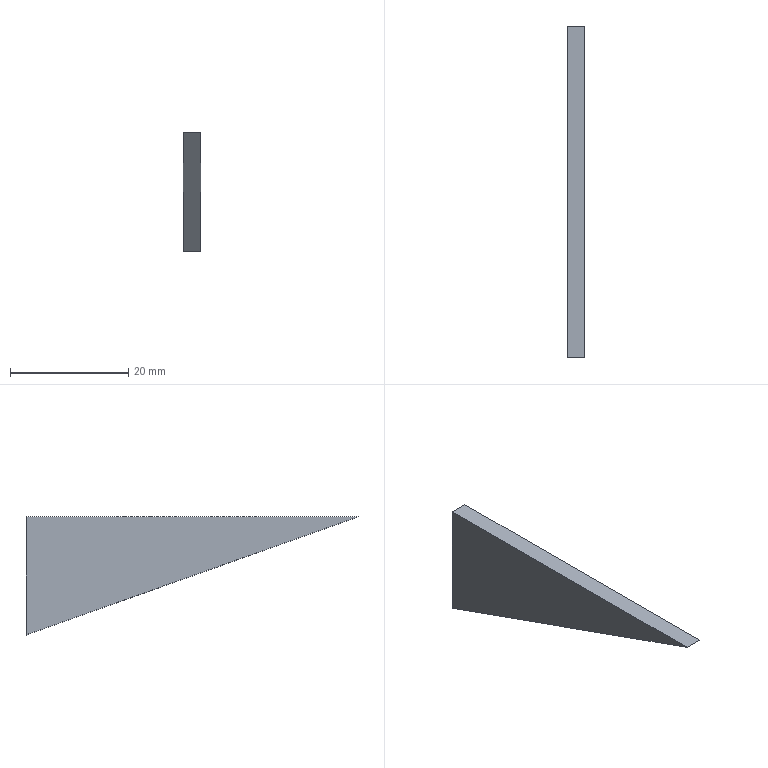Part | STEP file | 1 solid | 5 faces | box 3 x 56.217 x 20 mm | volume 1687 mm3 | plane 5
STEP:
#1=CARTESIAN_POINT('',(0.,0.,0.));
#2=DIRECTION('',(0.,0.,1.));
#3=DIRECTION('',(1.,0.,0.));
#4=AXIS2_PLACEMENT_3D('',#1,#2,#3);
#5=CARTESIAN_POINT('',(365.177,734.79,117.013));
#6=VERTEX_POINT('',#5);
#7=CARTESIAN_POINT('',(365.177,734.79,137.013));
#8=VERTEX_POINT('',#7);
#9=CARTESIAN_POINT('',(365.177,734.79,137.013));
#10=DIRECTION('',(0.,0.,1.));
#11=VECTOR('',#10,1.);
#12=LINE('',#9,#11);
#13=CARTESIAN_POINT('',(362.177,734.79,137.013));
#14=DIRECTION('',(0.,1.,0.));
#15=DIRECTION('',(0.,0.,1.));
#16=AXIS2_PLACEMENT_3D('',#13,#14,#15);
#17=PLANE('',#16);
#18=CARTESIAN_POINT('',(0.,3.));
#19=DIRECTION('',(1.,0.));
#20=VECTOR('',#19,1.);
#21=LINE('',#18,#20);
#22=(GEOMETRIC_REPRESENTATION_CONTEXT(2)PARAMETRIC_REPRESENTATION_CONTEXT()REPRESENTATION_CONTEXT('',''));
#23=DEFINITIONAL_REPRESENTATION('',(#21),#22);
#24=PCURVE('',#17,#23);
#25=CARTESIAN_POINT('',(365.177,0.,0.));
#26=DIRECTION('',(1.,0.,0.));
#27=DIRECTION('',(0.,0.,-1.));
#28=AXIS2_PLACEMENT_3D('',#25,#26,#27);
#29=PLANE('',#28);
#30=CARTESIAN_POINT('',(-137.013,734.79));
#31=DIRECTION('',(-1.,0.));
#32=VECTOR('',#31,1.);
#33=LINE('',#30,#32);
#34=(GEOMETRIC_REPRESENTATION_CONTEXT(2)PARAMETRIC_REPRESENTATION_CONTEXT()REPRESENTATION_CONTEXT('',''));
#35=DEFINITIONAL_REPRESENTATION('',(#33),#34);
#36=PCURVE('',#29,#35);
#37=SURFACE_CURVE('',#12,(#24,#36),.PCURVE_S1.);
#38=EDGE_CURVE('',#6,#8,#37,.T.);
#39=ORIENTED_EDGE('',*,*,#38,.F.);
#40=CARTESIAN_POINT('',(362.177,734.79,117.013));
#41=VERTEX_POINT('',#40);
#42=CARTESIAN_POINT('',(362.177,734.79,117.013));
#43=DIRECTION('',(1.,0.,0.));
#44=VECTOR('',#43,1.);
#45=LINE('',#42,#44);
#46=CARTESIAN_POINT('',(-20.,0.));
#47=DIRECTION('',(0.,1.));
#48=VECTOR('',#47,1.);
#49=LINE('',#46,#48);
#50=(GEOMETRIC_REPRESENTATION_CONTEXT(2)PARAMETRIC_REPRESENTATION_CONTEXT()REPRESENTATION_CONTEXT('',''));
#51=DEFINITIONAL_REPRESENTATION('',(#49),#50);
#52=PCURVE('',#17,#51);
#53=CARTESIAN_POINT('',(362.177,734.79,117.013));
#54=DIRECTION('',(0.,-0.3352,-0.9422));
#55=DIRECTION('',(0.,0.9422,-0.3352));
#56=AXIS2_PLACEMENT_3D('',#53,#54,#55);
#57=PLANE('',#56);
#58=CARTESIAN_POINT('',(0.,0.));
#59=DIRECTION('',(0.,1.));
#60=VECTOR('',#59,1.);
#61=LINE('',#58,#60);
#62=(GEOMETRIC_REPRESENTATION_CONTEXT(2)PARAMETRIC_REPRESENTATION_CONTEXT()REPRESENTATION_CONTEXT('',''));
#63=DEFINITIONAL_REPRESENTATION('',(#61),#62);
#64=PCURVE('',#57,#63);
#65=SURFACE_CURVE('',#45,(#52,#64),.PCURVE_S1.);
#66=EDGE_CURVE('',#41,#6,#65,.T.);
#67=ORIENTED_EDGE('',*,*,#66,.F.);
#68=CARTESIAN_POINT('',(362.177,734.79,137.013));
#69=VERTEX_POINT('',#68);
#70=CARTESIAN_POINT('',(362.177,734.79,137.013));
#71=DIRECTION('',(0.,0.,1.));
#72=VECTOR('',#71,1.);
#73=LINE('',#70,#72);
#74=CARTESIAN_POINT('',(0.,0.));
#75=DIRECTION('',(1.,0.));
#76=VECTOR('',#75,1.);
#77=LINE('',#74,#76);
#78=(GEOMETRIC_REPRESENTATION_CONTEXT(2)PARAMETRIC_REPRESENTATION_CONTEXT()REPRESENTATION_CONTEXT('',''));
#79=DEFINITIONAL_REPRESENTATION('',(#77),#78);
#80=PCURVE('',#17,#79);
#81=CARTESIAN_POINT('',(362.177,0.,0.));
#82=DIRECTION('',(1.,0.,0.));
#83=DIRECTION('',(0.,0.,-1.));
#84=AXIS2_PLACEMENT_3D('',#81,#82,#83);
#85=PLANE('',#84);
#86=CARTESIAN_POINT('',(-137.013,734.79));
#87=DIRECTION('',(-1.,0.));
#88=VECTOR('',#87,1.);
#89=LINE('',#86,#88);
#90=(GEOMETRIC_REPRESENTATION_CONTEXT(2)PARAMETRIC_REPRESENTATION_CONTEXT()REPRESENTATION_CONTEXT('',''));
#91=DEFINITIONAL_REPRESENTATION('',(#89),#90);
#92=PCURVE('',#85,#91);
#93=SURFACE_CURVE('',#73,(#80,#92),.PCURVE_S1.);
#94=EDGE_CURVE('',#41,#69,#93,.T.);
#95=ORIENTED_EDGE('',*,*,#94,.T.);
#96=CARTESIAN_POINT('',(362.177,734.79,137.013));
#97=DIRECTION('',(1.,0.,0.));
#98=VECTOR('',#97,1.);
#99=LINE('',#96,#98);
#100=CARTESIAN_POINT('',(0.,0.));
#101=DIRECTION('',(0.,1.));
#102=VECTOR('',#101,1.);
#103=LINE('',#100,#102);
#104=(GEOMETRIC_REPRESENTATION_CONTEXT(2)PARAMETRIC_REPRESENTATION_CONTEXT()REPRESENTATION_CONTEXT('',''));
#105=DEFINITIONAL_REPRESENTATION('',(#103),#104);
#106=PCURVE('',#17,#105);
#107=CARTESIAN_POINT('',(362.177,678.573,137.013));
#108=DIRECTION('',(0.,0.,1.));
#109=DIRECTION('',(1.,0.,0.));
#110=AXIS2_PLACEMENT_3D('',#107,#108,#109);
#111=PLANE('',#110);
#112=CARTESIAN_POINT('',(0.,56.217));
#113=DIRECTION('',(1.,0.));
#114=VECTOR('',#113,1.);
#115=LINE('',#112,#114);
#116=(GEOMETRIC_REPRESENTATION_CONTEXT(2)PARAMETRIC_REPRESENTATION_CONTEXT()REPRESENTATION_CONTEXT('',''));
#117=DEFINITIONAL_REPRESENTATION('',(#115),#116);
#118=PCURVE('',#111,#117);
#119=SURFACE_CURVE('',#99,(#106,#118),.PCURVE_S1.);
#120=EDGE_CURVE('',#69,#8,#119,.T.);
#121=ORIENTED_EDGE('',*,*,#120,.T.);
#122=EDGE_LOOP('',(#39,#67,#95,#121));
#123=FACE_BOUND('',#122,.T.);
#124=ADVANCED_FACE('',(#123),#17,.T.);
#125=CARTESIAN_POINT('',(365.177,678.573,137.013));
#126=VERTEX_POINT('',#125);
#127=CARTESIAN_POINT('',(365.177,734.79,117.013));
#128=DIRECTION('',(0.,0.9422,-0.3352));
#129=VECTOR('',#128,1.);
#130=LINE('',#127,#129);
#131=CARTESIAN_POINT('',(0.,3.));
#132=DIRECTION('',(1.,0.));
#133=VECTOR('',#132,1.);
#134=LINE('',#131,#133);
#135=(GEOMETRIC_REPRESENTATION_CONTEXT(2)PARAMETRIC_REPRESENTATION_CONTEXT()REPRESENTATION_CONTEXT('',''));
#136=DEFINITIONAL_REPRESENTATION('',(#134),#135);
#137=PCURVE('',#57,#136);
#138=CARTESIAN_POINT('',(-117.013,734.79));
#139=DIRECTION('',(0.3352,0.9422));
#140=VECTOR('',#139,1.);
#141=LINE('',#138,#140);
#142=(GEOMETRIC_REPRESENTATION_CONTEXT(2)PARAMETRIC_REPRESENTATION_CONTEXT()REPRESENTATION_CONTEXT('',''));
#143=DEFINITIONAL_REPRESENTATION('',(#141),#142);
#144=PCURVE('',#29,#143);
#145=SURFACE_CURVE('',#130,(#137,#144),.PCURVE_S1.);
#146=EDGE_CURVE('',#126,#6,#145,.T.);
#147=ORIENTED_EDGE('',*,*,#146,.F.);
#148=CARTESIAN_POINT('',(362.177,678.573,137.013));
#149=VERTEX_POINT('',#148);
#150=CARTESIAN_POINT('',(362.177,678.573,137.013));
#151=DIRECTION('',(1.,0.,0.));
#152=VECTOR('',#151,1.);
#153=LINE('',#150,#152);
#154=CARTESIAN_POINT('',(-59.669,0.));
#155=DIRECTION('',(0.,1.));
#156=VECTOR('',#155,1.);
#157=LINE('',#154,#156);
#158=(GEOMETRIC_REPRESENTATION_CONTEXT(2)PARAMETRIC_REPRESENTATION_CONTEXT()REPRESENTATION_CONTEXT('',''));
#159=DEFINITIONAL_REPRESENTATION('',(#157),#158);
#160=PCURVE('',#57,#159);
#161=CARTESIAN_POINT('',(0.,0.));
#162=DIRECTION('',(1.,0.));
#163=VECTOR('',#162,1.);
#164=LINE('',#161,#163);
#165=(GEOMETRIC_REPRESENTATION_CONTEXT(2)PARAMETRIC_REPRESENTATION_CONTEXT()REPRESENTATION_CONTEXT('',''));
#166=DEFINITIONAL_REPRESENTATION('',(#164),#165);
#167=PCURVE('',#111,#166);
#168=SURFACE_CURVE('',#153,(#160,#167),.PCURVE_S1.);
#169=EDGE_CURVE('',#149,#126,#168,.T.);
#170=ORIENTED_EDGE('',*,*,#169,.F.);
#171=CARTESIAN_POINT('',(362.177,734.79,117.013));
#172=DIRECTION('',(0.,0.9422,-0.3352));
#173=VECTOR('',#172,1.);
#174=LINE('',#171,#173);
#175=CARTESIAN_POINT('',(0.,0.));
#176=DIRECTION('',(1.,0.));
#177=VECTOR('',#176,1.);
#178=LINE('',#175,#177);
#179=(GEOMETRIC_REPRESENTATION_CONTEXT(2)PARAMETRIC_REPRESENTATION_CONTEXT()REPRESENTATION_CONTEXT('',''));
#180=DEFINITIONAL_REPRESENTATION('',(#178),#179);
#181=PCURVE('',#57,#180);
#182=CARTESIAN_POINT('',(-117.013,734.79));
#183=DIRECTION('',(0.3352,0.9422));
#184=VECTOR('',#183,1.);
#185=LINE('',#182,#184);
#186=(GEOMETRIC_REPRESENTATION_CONTEXT(2)PARAMETRIC_REPRESENTATION_CONTEXT()REPRESENTATION_CONTEXT('',''));
#187=DEFINITIONAL_REPRESENTATION('',(#185),#186);
#188=PCURVE('',#85,#187);
#189=SURFACE_CURVE('',#174,(#181,#188),.PCURVE_S1.);
#190=EDGE_CURVE('',#149,#41,#189,.T.);
#191=ORIENTED_EDGE('',*,*,#190,.T.);
#192=ORIENTED_EDGE('',*,*,#66,.T.);
#193=EDGE_LOOP('',(#147,#170,#191,#192));
#194=FACE_BOUND('',#193,.T.);
#195=ADVANCED_FACE('',(#194),#57,.T.);
#196=CARTESIAN_POINT('',(365.177,678.573,137.013));
#197=DIRECTION('',(0.,-1.,0.));
#198=VECTOR('',#197,1.);
#199=LINE('',#196,#198);
#200=CARTESIAN_POINT('',(3.,0.));
#201=DIRECTION('',(0.,-1.));
#202=VECTOR('',#201,1.);
#203=LINE('',#200,#202);
#204=(GEOMETRIC_REPRESENTATION_CONTEXT(2)PARAMETRIC_REPRESENTATION_CONTEXT()REPRESENTATION_CONTEXT('',''));
#205=DEFINITIONAL_REPRESENTATION('',(#203),#204);
#206=PCURVE('',#111,#205);
#207=CARTESIAN_POINT('',(-137.013,678.573));
#208=DIRECTION('',(0.,-1.));
#209=VECTOR('',#208,1.);
#210=LINE('',#207,#209);
#211=(GEOMETRIC_REPRESENTATION_CONTEXT(2)PARAMETRIC_REPRESENTATION_CONTEXT()REPRESENTATION_CONTEXT('',''));
#212=DEFINITIONAL_REPRESENTATION('',(#210),#211);
#213=PCURVE('',#29,#212);
#214=SURFACE_CURVE('',#199,(#206,#213),.PCURVE_S1.);
#215=EDGE_CURVE('',#8,#126,#214,.T.);
#216=ORIENTED_EDGE('',*,*,#215,.F.);
#217=ORIENTED_EDGE('',*,*,#120,.F.);
#218=CARTESIAN_POINT('',(362.177,678.573,137.013));
#219=DIRECTION('',(0.,-1.,0.));
#220=VECTOR('',#219,1.);
#221=LINE('',#218,#220);
#222=CARTESIAN_POINT('',(0.,0.));
#223=DIRECTION('',(0.,-1.));
#224=VECTOR('',#223,1.);
#225=LINE('',#222,#224);
#226=(GEOMETRIC_REPRESENTATION_CONTEXT(2)PARAMETRIC_REPRESENTATION_CONTEXT()REPRESENTATION_CONTEXT('',''));
#227=DEFINITIONAL_REPRESENTATION('',(#225),#226);
#228=PCURVE('',#111,#227);
#229=CARTESIAN_POINT('',(-137.013,678.573));
#230=DIRECTION('',(0.,-1.));
#231=VECTOR('',#230,1.);
#232=LINE('',#229,#231);
#233=(GEOMETRIC_REPRESENTATION_CONTEXT(2)PARAMETRIC_REPRESENTATION_CONTEXT()REPRESENTATION_CONTEXT('',''));
#234=DEFINITIONAL_REPRESENTATION('',(#232),#233);
#235=PCURVE('',#85,#234);
#236=SURFACE_CURVE('',#221,(#228,#235),.PCURVE_S1.);
#237=EDGE_CURVE('',#69,#149,#236,.T.);
#238=ORIENTED_EDGE('',*,*,#237,.T.);
#239=ORIENTED_EDGE('',*,*,#169,.T.);
#240=EDGE_LOOP('',(#216,#217,#238,#239));
#241=FACE_BOUND('',#240,.T.);
#242=ADVANCED_FACE('',(#241),#111,.T.);
#243=ORIENTED_EDGE('',*,*,#94,.F.);
#244=ORIENTED_EDGE('',*,*,#190,.F.);
#245=ORIENTED_EDGE('',*,*,#237,.F.);
#246=EDGE_LOOP('',(#243,#244,#245));
#247=FACE_BOUND('',#246,.T.);
#248=ADVANCED_FACE('',(#247),#85,.F.);
#249=ORIENTED_EDGE('',*,*,#38,.T.);
#250=ORIENTED_EDGE('',*,*,#215,.T.);
#251=ORIENTED_EDGE('',*,*,#146,.T.);
#252=EDGE_LOOP('',(#249,#250,#251));
#253=FACE_BOUND('',#252,.T.);
#254=ADVANCED_FACE('',(#253),#29,.T.);
#255=CLOSED_SHELL('',(#124,#195,#242,#248,#254));
#256=MANIFOLD_SOLID_BREP('',#255);
#257=(LENGTH_UNIT()NAMED_UNIT(*)SI_UNIT(.MILLI.,.METRE.));
#258=UNCERTAINTY_MEASURE_WITH_UNIT(LENGTH_MEASURE(0.0000001),#257,'','');
#259=(NAMED_UNIT(*)PLANE_ANGLE_UNIT()SI_UNIT($,.RADIAN.));
#260=(NAMED_UNIT(*)SI_UNIT($,.STERADIAN.)SOLID_ANGLE_UNIT());
#261=(GEOMETRIC_REPRESENTATION_CONTEXT(3)GLOBAL_UNCERTAINTY_ASSIGNED_CONTEXT((#258))GLOBAL_UNIT_ASSIGNED_CONTEXT((#257,#259,#260))REPRESENTATION_CONTEXT('',''));
#262=ADVANCED_BREP_SHAPE_REPRESENTATION('',(#4,#256),#261);